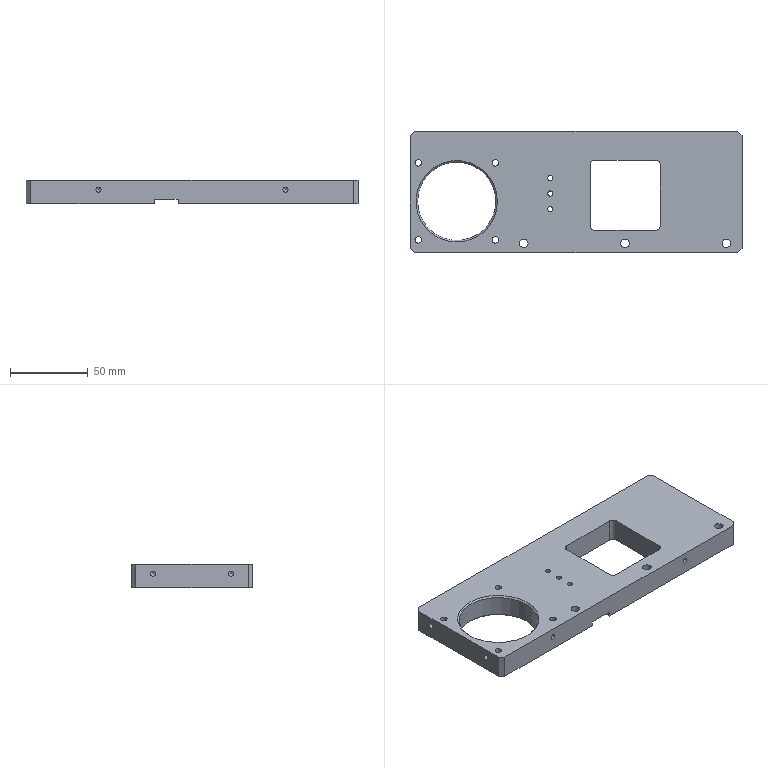CAM job | NX | 3-axis milling, drilling | part box 213 x 78 x 15 mm | stock box 218 x 83 x 20 mm
Tools:
number,name,description,diameter,corner_radius,flute_length,length,flutes
6,D6,平底铣刀-粗,6.0,0.0,25.0,75.0,2
9,D10,平底铣刀-粗,10.0,0.0,35.0,75.0,2
7,D6-J,平底铣刀-精,6.0,0.0,25.0,75.0,2
10,D10-J,平底铣刀-精,10.0,0.0,35.0,75.0,2
1,D80R0.8飞刀,圆鼻刀-粗,80.0,0.8,50.0,75.0,2
1,D80R0.8飞刀-J,圆鼻刀-精,80.0,0.8,50.0,75.0,2
2,D6倒角刀,倒角刀,6.0,0.0,3.0,25.0,2
21,M4X0.7,丝锥,3.3,0.0,35.0,50.0,2
22,M5X0.8,丝锥,4.2,0.0,35.0,50.0,2
17,ZT5.5,钻头,5.5,0.0,35.0,50.0,2
13,钻头3.3,Twist Drill 3.3 mm,3.3,0.0,35.0,35.008,2
14,钻头4.2,Twist Drill 4.2 mm,4.2,0.0,41.0,41.738,2
Operations:
program,operation,operation_type,tool,method,geometry_group,spindle_rpm,surface_speed,feed_per_tooth,feed_cut,feed_plunge,cut_length_mm,path_length_mm,cut_time_min,machine_time_min
B,底壁铣飞面开粗_COPY,VolumeBased25DMillingOperation,D80R0.8飞刀,分层开粗-切深K-步距G,W-B,2800.0,703.696,0.5357,3000.0,100.0,5676.277,5890.875,1.892,1.914
B,底壁铣飞面精光_COPY,VolumeBased25DMillingOperation,D80R0.8飞刀-J,侧刃精光-切深K-步距G,W-B,4000.0,1005.28,0.125,1000.0,100.0,630.11,666.11,0.6301,0.6337
B,封闭铣廓倒角6X45L_COPY,PlanarMilling,D6倒角刀,爬面_倒角-切深0-步距G,W-B,7000.0,131.0,0.1071,1500.0,100.0,349.285,492.849,0.2329,0.2472
B,钻倒角_2,Operation,D6倒角刀,METHOD,W-B,8000.0,150.796,0.0625,1000.0,0.0,15.6,98.081,0.0156,0.0238
B,钻倒角_3,Operation,D6倒角刀,METHOD,W-B,8000.0,150.796,0.0625,1000.0,0.0,22.8,243.365,0.0228,0.0449
B,平面去毛刺6X45L_COPY,SurfaceContour,D6倒角刀,爬面_倒角-切深0-步距G,W-B,6500.0,122.519,0.1154,1500.0,100.0,869.677,1563.376,0.5798,0.6492
B,底壁铣倒角_COPY,VolumeBased25DMillingOperation,D6倒角刀,爬面_倒角-切深0-步距G,W-B,6500.0,122.519,0.1154,1500.0,100.0,160.856,201.256,0.1072,0.1113
A,顶面,FaceMilling,D80R0.8飞刀,侧刃精光-切深K-步距G,W-A,4000.0,1005.31,0.125,1000.0,100.0,652.667,688.667,0.6527,0.6563
A,外形粗_2,VolumeBased25DMillingOperation,D10,METHOD,W-A,8000.0,251.327,0.3125,5000.0,80.0,12748.821,12802.321,2.55,2.555
A,底壁粗_1,VolumeBased25DMillingOperation,D10,METHOD,W-A,6000.0,113.0,0.2083,3500.0,100.0,1070.4,1155.621,0.3058,0.3144
A,框开粗_1,VolumeBased25DMillingOperation,D10,METHOD,W-A,6000.0,188.0,0.25,4000.0,80.0,8488.749,8703.054,2.122,2.144
A,打点-深0.8,Operation,D6倒角刀,NONE,W-A,8000.0,150.796,0.0312,500.0,90.0,18.0,426.629,0.036,0.0769
A,打点0.8,Operation,D6倒角刀,METHOD,W-A,8000.0,150.796,0.0312,500.0,0.0,1.8,43.6,0.0036,0.0078
A,通孔-M4螺纹底孔,Operation,钻头3.3,NONE,W-A,3000.0,31.102,0.05,300.0,90.0,56.974,182.048,0.1899,0.2024
A,通孔-M5螺纹底孔,Operation,钻头4.2,NONE,W-A,3000.0,39.584,0.0583,350.0,90.0,93.047,377.617,0.2658,0.2943
A,沉头孔-钻孔0段,Operation,ZT5.5,NONE,W-A,1200.0,20.735,0.0625,150.0,90.0,58.957,289.93,0.393,0.4161
A,铣孔开粗D6_1,CylinderMilling,D6,NONE,W-A,8000.0,150.796,0.075,1200.0,100.0,476.699,806.399,0.3972,0.4302
A,铣孔精光D6_1,CylinderMilling,D6-J,精光步距切深关,W-A,8000.0,150.796,0.0312,500.0,100.0,100.196,431.396,0.2004,0.2335
A,清角D4,ZLevelMilling,D6-J,METHOD,W-A,6000.0,75.0,0.25,2500.0,80.0,1710.425,1922.526,0.6848,0.706
A,底侧精_3,VolumeBased25DMillingOperation,D6-J,METHOD,W-A,6000.0,113.0,0.2083,1200.0,100.0,175.483,272.363,0.1462,0.1559
A,底精_1,VolumeBased25DMillingOperation,D6-J,METHOD,W-A,6000.0,113.0,0.2083,1200.0,100.0,342.233,387.233,0.2852,0.2897
A,框半精_1,VolumeBased25DMillingOperation,D6-J,METHOD,W-A,6000.0,113.0,0.0833,1000.0,100.0,610.606,872.201,0.6106,0.6368
A,框精_1,VolumeBased25DMillingOperation,D6-J,METHOD,W-A,6000.0,113.0,0.0833,1000.0,100.0,304.903,567.279,0.3049,0.3311
A,仅选体,SurfaceContour,D6倒角刀,METHOD,W-A,8000.0,150.796,0.1875,3000.0,100.0,956.847,1347.645,0.3189,0.358
A,钻倒角_1,Operation,D6倒角刀,METHOD,W-A,8000.0,150.796,0.0312,500.0,0.0,15.6,104.081,0.0312,0.04
A,铣倒角_1,PlanarMilling,D6倒角刀,METHOD,W-A,8000.0,150.796,0.0312,500.0,100.0,72.081,384.593,0.1442,0.1754
A,铣倒角_2,PlanarMilling,D6倒角刀,NONE,W-A,8000.0,150.796,0.05,800.0,100.0,120.753,372.813,0.1509,0.1761
A,铣倒角_3,PlanarMilling,D6倒角刀,METHOD,W-A,8000.0,150.796,0.05,800.0,100.0,159.022,202.022,0.1988,0.2031
A,铣倒角_3_COPY,PlanarMilling,D6倒角刀,METHOD,W-A,8000.0,150.796,0.05,800.0,100.0,162.164,205.164,0.2027,0.207
A,通孔-攻牙M5,Operation,M5X0.8,METHOD,W-A,500.0,6.597,0.0008,0.8,90.0,78.0,347.523,97.5,97.527
A,通孔-攻牙M4,Operation,M4X0.7,METHOD,W-A,600.0,6.22,0.0006,0.7,90.0,48.0,164.1,68.571,68.583
A,外形半精_2,VolumeBased25DMillingOperation,D10-J,METHOD,W-A,8000.0,251.327,0.0625,1000.0,100.0,611.345,680.345,0.6113,0.6182